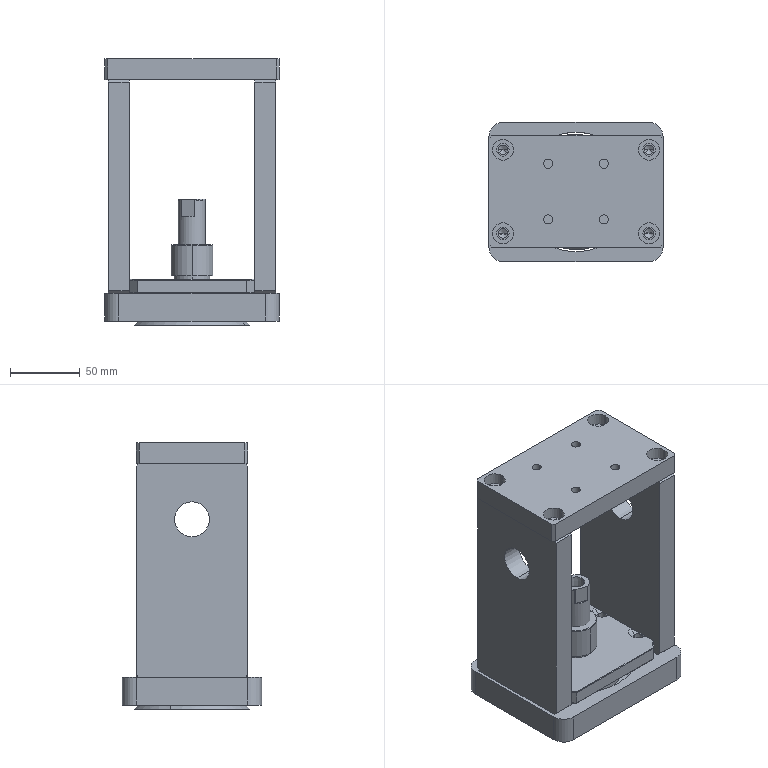Part | SolidWorks | 7 solids | 246 faces | box 125 x 100 x 191.5 mm | volume 742164 mm3 | cylinder 122 | plane 79 | cone 45 | commonest cylinder face diameters 6.6 x16 6.8 x16 15 x16 8.5 x10 5 x8 9 x8